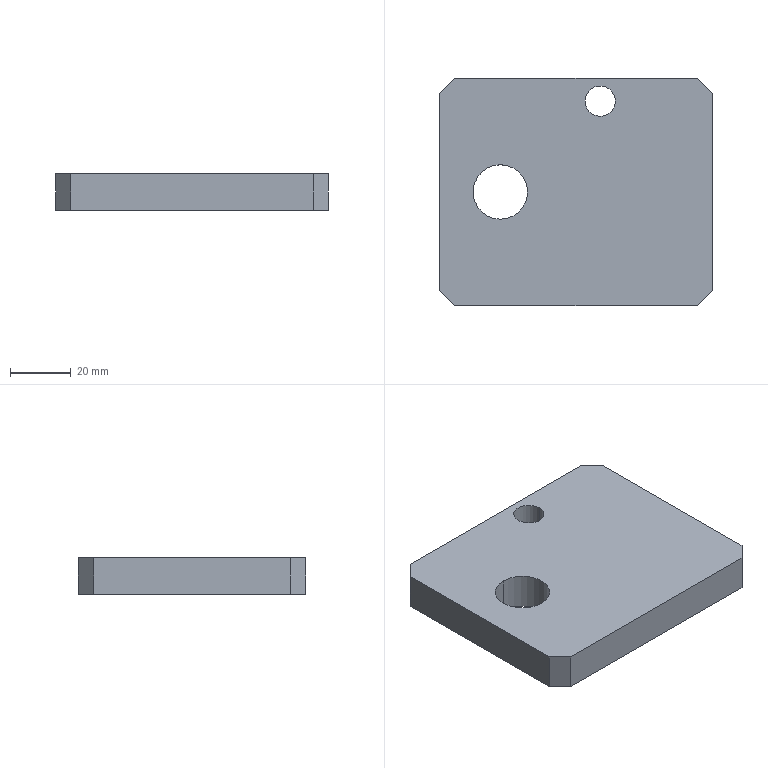Part | STEP file | [18] | 1 solid | 14 faces | box 90 x 75 x 12 mm | volume 76404 mm3 | plane 10 | cylinder 4 | commonest cylinder face diameters 10 x2 18 x2
STEP:
#1=CARTESIAN_POINT('',(20.,46.5,12.));
#2=VERTEX_POINT('',#1);
#3=CARTESIAN_POINT('',(20.,28.5,12.));
#4=VERTEX_POINT('',#3);
#5=CARTESIAN_POINT('',(20.,37.5,12.));
#6=DIRECTION('',(0.,0.,-1.));
#7=DIRECTION('',(0.,-1.,0.));
#8=AXIS2_PLACEMENT_3D('',#5,#6,#7);
#9=CIRCLE('',#8,9.);
#10=EDGE_CURVE('',#2,#4,#9,.T.);
#11=ORIENTED_EDGE('',*,*,#10,.F.);
#12=CARTESIAN_POINT('',(20.,46.5,0.));
#13=VERTEX_POINT('',#12);
#14=CARTESIAN_POINT('',(20.,46.5,12.));
#15=DIRECTION('',(0.,0.,-1.));
#16=VECTOR('',#15,1000.);
#17=LINE('',#14,#16);
#18=EDGE_CURVE('',#2,#13,#17,.T.);
#19=ORIENTED_EDGE('',*,*,#18,.T.);
#20=CARTESIAN_POINT('',(20.,28.5,0.));
#21=VERTEX_POINT('',#20);
#22=CARTESIAN_POINT('',(20.,37.5,0.));
#23=DIRECTION('',(0.,0.,1.));
#24=DIRECTION('',(0.,1.,0.));
#25=AXIS2_PLACEMENT_3D('',#22,#23,#24);
#26=CIRCLE('',#25,9.);
#27=EDGE_CURVE('',#21,#13,#26,.T.);
#28=ORIENTED_EDGE('',*,*,#27,.F.);
#29=CARTESIAN_POINT('',(20.,28.5,12.));
#30=DIRECTION('',(0.,0.,-1.));
#31=VECTOR('',#30,1000.);
#32=LINE('',#29,#31);
#33=EDGE_CURVE('',#4,#21,#32,.T.);
#34=ORIENTED_EDGE('',*,*,#33,.F.);
#35=EDGE_LOOP('',(#11,#19,#28,#34));
#36=FACE_OUTER_BOUND('',#35,.T.);
#37=CARTESIAN_POINT('',(20.,37.5,12.));
#38=DIRECTION('',(0.,0.,-1.));
#39=DIRECTION('',(0.,-1.,0.));
#40=AXIS2_PLACEMENT_3D('',#37,#38,#39);
#41=CYLINDRICAL_SURFACE('',#40,9.);
#42=ADVANCED_FACE('',(#36),#41,.F.);
#43=CARTESIAN_POINT('',(58.,67.5,0.));
#44=VERTEX_POINT('',#43);
#45=CARTESIAN_POINT('',(48.,67.5,0.));
#46=VERTEX_POINT('',#45);
#47=CARTESIAN_POINT('',(53.,67.5,0.));
#48=DIRECTION('',(0.,0.,1.));
#49=DIRECTION('',(-1.,0.,0.));
#50=AXIS2_PLACEMENT_3D('',#47,#48,#49);
#51=CIRCLE('',#50,5.);
#52=EDGE_CURVE('',#44,#46,#51,.T.);
#53=ORIENTED_EDGE('',*,*,#52,.F.);
#54=CARTESIAN_POINT('',(58.,67.5,12.));
#55=VERTEX_POINT('',#54);
#56=CARTESIAN_POINT('',(58.,67.5,0.));
#57=DIRECTION('',(0.,0.,1.));
#58=VECTOR('',#57,1000.);
#59=LINE('',#56,#58);
#60=EDGE_CURVE('',#44,#55,#59,.T.);
#61=ORIENTED_EDGE('',*,*,#60,.T.);
#62=CARTESIAN_POINT('',(48.,67.5,12.));
#63=VERTEX_POINT('',#62);
#64=CARTESIAN_POINT('',(53.,67.5,12.));
#65=DIRECTION('',(0.,0.,-1.));
#66=DIRECTION('',(1.,0.,0.));
#67=AXIS2_PLACEMENT_3D('',#64,#65,#66);
#68=CIRCLE('',#67,5.);
#69=EDGE_CURVE('',#63,#55,#68,.T.);
#70=ORIENTED_EDGE('',*,*,#69,.F.);
#71=CARTESIAN_POINT('',(48.,67.5,0.));
#72=DIRECTION('',(0.,0.,1.));
#73=VECTOR('',#72,1000.);
#74=LINE('',#71,#73);
#75=EDGE_CURVE('',#46,#63,#74,.T.);
#76=ORIENTED_EDGE('',*,*,#75,.F.);
#77=EDGE_LOOP('',(#53,#61,#70,#76));
#78=FACE_OUTER_BOUND('',#77,.T.);
#79=CARTESIAN_POINT('',(53.,67.5,0.));
#80=DIRECTION('',(0.,0.,1.));
#81=DIRECTION('',(-1.,0.,0.));
#82=AXIS2_PLACEMENT_3D('',#79,#80,#81);
#83=CYLINDRICAL_SURFACE('',#82,5.);
#84=ADVANCED_FACE('',(#78),#83,.F.);
#85=CARTESIAN_POINT('',(20.,37.5,12.));
#86=DIRECTION('',(0.,0.,-1.));
#87=DIRECTION('',(0.,-1.,0.));
#88=AXIS2_PLACEMENT_3D('',#85,#86,#87);
#89=CIRCLE('',#88,9.);
#90=EDGE_CURVE('',#4,#2,#89,.T.);
#91=ORIENTED_EDGE('',*,*,#90,.T.);
#92=ORIENTED_EDGE('',*,*,#10,.T.);
#93=EDGE_LOOP('',(#91,#92));
#94=FACE_BOUND('',#93,.T.);
#95=ORIENTED_EDGE('',*,*,#69,.T.);
#96=CARTESIAN_POINT('',(53.,67.5,12.));
#97=DIRECTION('',(0.,0.,-1.));
#98=DIRECTION('',(1.,0.,0.));
#99=AXIS2_PLACEMENT_3D('',#96,#97,#98);
#100=CIRCLE('',#99,5.);
#101=EDGE_CURVE('',#55,#63,#100,.T.);
#102=ORIENTED_EDGE('',*,*,#101,.T.);
#103=EDGE_LOOP('',(#95,#102));
#104=FACE_BOUND('',#103,.T.);
#105=CARTESIAN_POINT('',(5.,75.,12.));
#106=VERTEX_POINT('',#105);
#107=CARTESIAN_POINT('',(85.,75.,12.));
#108=VERTEX_POINT('',#107);
#109=CARTESIAN_POINT('',(45.,75.,12.));
#110=DIRECTION('',(1.,0.,0.));
#111=VECTOR('',#110,1000.);
#112=LINE('',#109,#111);
#113=EDGE_CURVE('',#106,#108,#112,.T.);
#114=ORIENTED_EDGE('',*,*,#113,.F.);
#115=CARTESIAN_POINT('',(0.,70.,12.));
#116=VERTEX_POINT('',#115);
#117=CARTESIAN_POINT('',(6.25,76.25,12.));
#118=DIRECTION('',(-0.7071,-0.7071,0.));
#119=VECTOR('',#118,1000.);
#120=LINE('',#117,#119);
#121=EDGE_CURVE('',#106,#116,#120,.T.);
#122=ORIENTED_EDGE('',*,*,#121,.T.);
#123=CARTESIAN_POINT('',(0.,5.,12.));
#124=VERTEX_POINT('',#123);
#125=CARTESIAN_POINT('',(0.,37.5,12.));
#126=DIRECTION('',(0.,1.,0.));
#127=VECTOR('',#126,1000.);
#128=LINE('',#125,#127);
#129=EDGE_CURVE('',#124,#116,#128,.T.);
#130=ORIENTED_EDGE('',*,*,#129,.F.);
#131=CARTESIAN_POINT('',(5.,0.,12.));
#132=VERTEX_POINT('',#131);
#133=CARTESIAN_POINT('',(6.25,-1.25,12.));
#134=DIRECTION('',(0.7071,-0.7071,0.));
#135=VECTOR('',#134,1000.);
#136=LINE('',#133,#135);
#137=EDGE_CURVE('',#124,#132,#136,.T.);
#138=ORIENTED_EDGE('',*,*,#137,.T.);
#139=CARTESIAN_POINT('',(85.,0.,12.));
#140=VERTEX_POINT('',#139);
#141=CARTESIAN_POINT('',(45.,0.,12.));
#142=DIRECTION('',(-1.,0.,0.));
#143=VECTOR('',#142,1000.);
#144=LINE('',#141,#143);
#145=EDGE_CURVE('',#140,#132,#144,.T.);
#146=ORIENTED_EDGE('',*,*,#145,.F.);
#147=CARTESIAN_POINT('',(90.,5.,12.));
#148=VERTEX_POINT('',#147);
#149=CARTESIAN_POINT('',(83.75,-1.25,12.));
#150=DIRECTION('',(0.7071,0.7071,0.));
#151=VECTOR('',#150,1000.);
#152=LINE('',#149,#151);
#153=EDGE_CURVE('',#140,#148,#152,.T.);
#154=ORIENTED_EDGE('',*,*,#153,.T.);
#155=CARTESIAN_POINT('',(90.,70.,12.));
#156=VERTEX_POINT('',#155);
#157=CARTESIAN_POINT('',(90.,37.5,12.));
#158=DIRECTION('',(0.,-1.,0.));
#159=VECTOR('',#158,1000.);
#160=LINE('',#157,#159);
#161=EDGE_CURVE('',#156,#148,#160,.T.);
#162=ORIENTED_EDGE('',*,*,#161,.F.);
#163=CARTESIAN_POINT('',(83.75,76.25,12.));
#164=DIRECTION('',(-0.7071,0.7071,0.));
#165=VECTOR('',#164,1000.);
#166=LINE('',#163,#165);
#167=EDGE_CURVE('',#156,#108,#166,.T.);
#168=ORIENTED_EDGE('',*,*,#167,.T.);
#169=EDGE_LOOP('',(#114,#122,#130,#138,#146,#154,#162,#168));
#170=FACE_OUTER_BOUND('',#169,.T.);
#171=CARTESIAN_POINT('',(45.,37.5,12.));
#172=DIRECTION('',(0.,0.,1.));
#173=DIRECTION('',(0.,1.,0.));
#174=AXIS2_PLACEMENT_3D('',#171,#172,#173);
#175=PLANE('',#174);
#176=ADVANCED_FACE('',(#94,#104,#170),#175,.T.);
#177=CARTESIAN_POINT('',(90.,5.,0.));
#178=VERTEX_POINT('',#177);
#179=CARTESIAN_POINT('',(90.,70.,0.));
#180=VERTEX_POINT('',#179);
#181=CARTESIAN_POINT('',(90.,37.5,0.));
#182=DIRECTION('',(0.,1.,0.));
#183=VECTOR('',#182,1000.);
#184=LINE('',#181,#183);
#185=EDGE_CURVE('',#178,#180,#184,.T.);
#186=ORIENTED_EDGE('',*,*,#185,.T.);
#187=CARTESIAN_POINT('',(90.,70.,0.));
#188=DIRECTION('',(0.,0.,1.));
#189=VECTOR('',#188,1000.);
#190=LINE('',#187,#189);
#191=EDGE_CURVE('',#180,#156,#190,.T.);
#192=ORIENTED_EDGE('',*,*,#191,.T.);
#193=ORIENTED_EDGE('',*,*,#161,.T.);
#194=CARTESIAN_POINT('',(90.,5.,0.));
#195=DIRECTION('',(0.,0.,-1.));
#196=VECTOR('',#195,1000.);
#197=LINE('',#194,#196);
#198=EDGE_CURVE('',#148,#178,#197,.T.);
#199=ORIENTED_EDGE('',*,*,#198,.T.);
#200=EDGE_LOOP('',(#186,#192,#193,#199));
#201=FACE_OUTER_BOUND('',#200,.T.);
#202=CARTESIAN_POINT('',(90.,37.5,0.));
#203=DIRECTION('',(1.,0.,0.));
#204=DIRECTION('',(0.,0.,-1.));
#205=AXIS2_PLACEMENT_3D('',#202,#203,#204);
#206=PLANE('',#205);
#207=ADVANCED_FACE('',(#201),#206,.T.);
#208=ORIENTED_EDGE('',*,*,#145,.T.);
#209=CARTESIAN_POINT('',(5.,0.,0.));
#210=VERTEX_POINT('',#209);
#211=CARTESIAN_POINT('',(5.,0.,0.));
#212=DIRECTION('',(0.,0.,-1.));
#213=VECTOR('',#212,1000.);
#214=LINE('',#211,#213);
#215=EDGE_CURVE('',#132,#210,#214,.T.);
#216=ORIENTED_EDGE('',*,*,#215,.T.);
#217=CARTESIAN_POINT('',(85.,0.,0.));
#218=VERTEX_POINT('',#217);
#219=CARTESIAN_POINT('',(45.,0.,0.));
#220=DIRECTION('',(1.,0.,0.));
#221=VECTOR('',#220,1000.);
#222=LINE('',#219,#221);
#223=EDGE_CURVE('',#210,#218,#222,.T.);
#224=ORIENTED_EDGE('',*,*,#223,.T.);
#225=CARTESIAN_POINT('',(85.,0.,0.));
#226=DIRECTION('',(0.,0.,1.));
#227=VECTOR('',#226,1000.);
#228=LINE('',#225,#227);
#229=EDGE_CURVE('',#218,#140,#228,.T.);
#230=ORIENTED_EDGE('',*,*,#229,.T.);
#231=EDGE_LOOP('',(#208,#216,#224,#230));
#232=FACE_OUTER_BOUND('',#231,.T.);
#233=CARTESIAN_POINT('',(45.,0.,0.));
#234=DIRECTION('',(0.,-1.,0.));
#235=DIRECTION('',(0.,0.,1.));
#236=AXIS2_PLACEMENT_3D('',#233,#234,#235);
#237=PLANE('',#236);
#238=ADVANCED_FACE('',(#232),#237,.T.);
#239=ORIENTED_EDGE('',*,*,#129,.T.);
#240=CARTESIAN_POINT('',(0.,70.,0.));
#241=VERTEX_POINT('',#240);
#242=CARTESIAN_POINT('',(0.,70.,0.));
#243=DIRECTION('',(0.,0.,-1.));
#244=VECTOR('',#243,1000.);
#245=LINE('',#242,#244);
#246=EDGE_CURVE('',#116,#241,#245,.T.);
#247=ORIENTED_EDGE('',*,*,#246,.T.);
#248=CARTESIAN_POINT('',(0.,5.,0.));
#249=VERTEX_POINT('',#248);
#250=CARTESIAN_POINT('',(0.,37.5,0.));
#251=DIRECTION('',(0.,-1.,0.));
#252=VECTOR('',#251,1000.);
#253=LINE('',#250,#252);
#254=EDGE_CURVE('',#241,#249,#253,.T.);
#255=ORIENTED_EDGE('',*,*,#254,.T.);
#256=CARTESIAN_POINT('',(0.,5.,0.));
#257=DIRECTION('',(0.,0.,1.));
#258=VECTOR('',#257,1000.);
#259=LINE('',#256,#258);
#260=EDGE_CURVE('',#249,#124,#259,.T.);
#261=ORIENTED_EDGE('',*,*,#260,.T.);
#262=EDGE_LOOP('',(#239,#247,#255,#261));
#263=FACE_OUTER_BOUND('',#262,.T.);
#264=CARTESIAN_POINT('',(0.,37.5,0.));
#265=DIRECTION('',(-1.,0.,0.));
#266=DIRECTION('',(0.,0.,1.));
#267=AXIS2_PLACEMENT_3D('',#264,#265,#266);
#268=PLANE('',#267);
#269=ADVANCED_FACE('',(#263),#268,.T.);
#270=ORIENTED_EDGE('',*,*,#27,.T.);
#271=CARTESIAN_POINT('',(20.,37.5,0.));
#272=DIRECTION('',(0.,0.,1.));
#273=DIRECTION('',(0.,1.,0.));
#274=AXIS2_PLACEMENT_3D('',#271,#272,#273);
#275=CIRCLE('',#274,9.);
#276=EDGE_CURVE('',#13,#21,#275,.T.);
#277=ORIENTED_EDGE('',*,*,#276,.T.);
#278=EDGE_LOOP('',(#270,#277));
#279=FACE_BOUND('',#278,.T.);
#280=CARTESIAN_POINT('',(53.,67.5,0.));
#281=DIRECTION('',(0.,0.,1.));
#282=DIRECTION('',(-1.,0.,0.));
#283=AXIS2_PLACEMENT_3D('',#280,#281,#282);
#284=CIRCLE('',#283,5.);
#285=EDGE_CURVE('',#46,#44,#284,.T.);
#286=ORIENTED_EDGE('',*,*,#285,.T.);
#287=ORIENTED_EDGE('',*,*,#52,.T.);
#288=EDGE_LOOP('',(#286,#287));
#289=FACE_BOUND('',#288,.T.);
#290=ORIENTED_EDGE('',*,*,#254,.F.);
#291=CARTESIAN_POINT('',(5.,75.,0.));
#292=VERTEX_POINT('',#291);
#293=CARTESIAN_POINT('',(6.25,76.25,0.));
#294=DIRECTION('',(0.7071,0.7071,0.));
#295=VECTOR('',#294,1000.);
#296=LINE('',#293,#295);
#297=EDGE_CURVE('',#241,#292,#296,.T.);
#298=ORIENTED_EDGE('',*,*,#297,.T.);
#299=CARTESIAN_POINT('',(85.,75.,0.));
#300=VERTEX_POINT('',#299);
#301=CARTESIAN_POINT('',(45.,75.,0.));
#302=DIRECTION('',(-1.,0.,0.));
#303=VECTOR('',#302,1000.);
#304=LINE('',#301,#303);
#305=EDGE_CURVE('',#300,#292,#304,.T.);
#306=ORIENTED_EDGE('',*,*,#305,.F.);
#307=CARTESIAN_POINT('',(83.75,76.25,0.));
#308=DIRECTION('',(0.7071,-0.7071,0.));
#309=VECTOR('',#308,1000.);
#310=LINE('',#307,#309);
#311=EDGE_CURVE('',#300,#180,#310,.T.);
#312=ORIENTED_EDGE('',*,*,#311,.T.);
#313=ORIENTED_EDGE('',*,*,#185,.F.);
#314=CARTESIAN_POINT('',(83.75,-1.25,0.));
#315=DIRECTION('',(-0.7071,-0.7071,0.));
#316=VECTOR('',#315,1000.);
#317=LINE('',#314,#316);
#318=EDGE_CURVE('',#178,#218,#317,.T.);
#319=ORIENTED_EDGE('',*,*,#318,.T.);
#320=ORIENTED_EDGE('',*,*,#223,.F.);
#321=CARTESIAN_POINT('',(6.25,-1.25,0.));
#322=DIRECTION('',(-0.7071,0.7071,0.));
#323=VECTOR('',#322,1000.);
#324=LINE('',#321,#323);
#325=EDGE_CURVE('',#210,#249,#324,.T.);
#326=ORIENTED_EDGE('',*,*,#325,.T.);
#327=EDGE_LOOP('',(#290,#298,#306,#312,#313,#319,#320,#326));
#328=FACE_OUTER_BOUND('',#327,.T.);
#329=CARTESIAN_POINT('',(45.,37.5,0.));
#330=DIRECTION('',(0.,0.,-1.));
#331=DIRECTION('',(0.,-1.,0.));
#332=AXIS2_PLACEMENT_3D('',#329,#330,#331);
#333=PLANE('',#332);
#334=ADVANCED_FACE('',(#279,#289,#328),#333,.T.);
#335=ORIENTED_EDGE('',*,*,#305,.T.);
#336=CARTESIAN_POINT('',(5.,75.,0.));
#337=DIRECTION('',(0.,0.,1.));
#338=VECTOR('',#337,1000.);
#339=LINE('',#336,#338);
#340=EDGE_CURVE('',#292,#106,#339,.T.);
#341=ORIENTED_EDGE('',*,*,#340,.T.);
#342=ORIENTED_EDGE('',*,*,#113,.T.);
#343=CARTESIAN_POINT('',(85.,75.,0.));
#344=DIRECTION('',(0.,0.,-1.));
#345=VECTOR('',#344,1000.);
#346=LINE('',#343,#345);
#347=EDGE_CURVE('',#108,#300,#346,.T.);
#348=ORIENTED_EDGE('',*,*,#347,.T.);
#349=EDGE_LOOP('',(#335,#341,#342,#348));
#350=FACE_OUTER_BOUND('',#349,.T.);
#351=CARTESIAN_POINT('',(45.,75.,0.));
#352=DIRECTION('',(0.,1.,0.));
#353=DIRECTION('',(0.,0.,-1.));
#354=AXIS2_PLACEMENT_3D('',#351,#352,#353);
#355=PLANE('',#354);
#356=ADVANCED_FACE('',(#350),#355,.T.);
#357=ORIENTED_EDGE('',*,*,#311,.F.);
#358=ORIENTED_EDGE('',*,*,#347,.F.);
#359=ORIENTED_EDGE('',*,*,#167,.F.);
#360=ORIENTED_EDGE('',*,*,#191,.F.);
#361=EDGE_LOOP('',(#357,#358,#359,#360));
#362=FACE_OUTER_BOUND('',#361,.T.);
#363=CARTESIAN_POINT('',(90.,70.,0.));
#364=DIRECTION('',(-0.7071,-0.7071,0.));
#365=DIRECTION('',(0.,0.,1.));
#366=AXIS2_PLACEMENT_3D('',#363,#364,#365);
#367=PLANE('',#366);
#368=ADVANCED_FACE('',(#362),#367,.F.);
#369=ORIENTED_EDGE('',*,*,#318,.F.);
#370=ORIENTED_EDGE('',*,*,#198,.F.);
#371=ORIENTED_EDGE('',*,*,#153,.F.);
#372=ORIENTED_EDGE('',*,*,#229,.F.);
#373=EDGE_LOOP('',(#369,#370,#371,#372));
#374=FACE_OUTER_BOUND('',#373,.T.);
#375=CARTESIAN_POINT('',(85.,0.,0.));
#376=DIRECTION('',(-0.7071,0.7071,0.));
#377=DIRECTION('',(0.,0.,1.));
#378=AXIS2_PLACEMENT_3D('',#375,#376,#377);
#379=PLANE('',#378);
#380=ADVANCED_FACE('',(#374),#379,.F.);
#381=ORIENTED_EDGE('',*,*,#297,.F.);
#382=ORIENTED_EDGE('',*,*,#246,.F.);
#383=ORIENTED_EDGE('',*,*,#121,.F.);
#384=ORIENTED_EDGE('',*,*,#340,.F.);
#385=EDGE_LOOP('',(#381,#382,#383,#384));
#386=FACE_OUTER_BOUND('',#385,.T.);
#387=CARTESIAN_POINT('',(5.,75.,0.));
#388=DIRECTION('',(0.7071,-0.7071,0.));
#389=DIRECTION('',(0.,0.,1.));
#390=AXIS2_PLACEMENT_3D('',#387,#388,#389);
#391=PLANE('',#390);
#392=ADVANCED_FACE('',(#386),#391,.F.);
#393=ORIENTED_EDGE('',*,*,#325,.F.);
#394=ORIENTED_EDGE('',*,*,#215,.F.);
#395=ORIENTED_EDGE('',*,*,#137,.F.);
#396=ORIENTED_EDGE('',*,*,#260,.F.);
#397=EDGE_LOOP('',(#393,#394,#395,#396));
#398=FACE_OUTER_BOUND('',#397,.T.);
#399=CARTESIAN_POINT('',(0.,5.,0.));
#400=DIRECTION('',(0.7071,0.7071,0.));
#401=DIRECTION('',(0.,0.,1.));
#402=AXIS2_PLACEMENT_3D('',#399,#400,#401);
#403=PLANE('',#402);
#404=ADVANCED_FACE('',(#398),#403,.F.);
#405=ORIENTED_EDGE('',*,*,#60,.F.);
#406=ORIENTED_EDGE('',*,*,#285,.F.);
#407=ORIENTED_EDGE('',*,*,#75,.T.);
#408=ORIENTED_EDGE('',*,*,#101,.F.);
#409=EDGE_LOOP('',(#405,#406,#407,#408));
#410=FACE_OUTER_BOUND('',#409,.T.);
#411=CARTESIAN_POINT('',(53.,67.5,0.));
#412=DIRECTION('',(0.,0.,1.));
#413=DIRECTION('',(-1.,0.,0.));
#414=AXIS2_PLACEMENT_3D('',#411,#412,#413);
#415=CYLINDRICAL_SURFACE('',#414,5.);
#416=ADVANCED_FACE('',(#410),#415,.F.);
#417=ORIENTED_EDGE('',*,*,#18,.F.);
#418=ORIENTED_EDGE('',*,*,#90,.F.);
#419=ORIENTED_EDGE('',*,*,#33,.T.);
#420=ORIENTED_EDGE('',*,*,#276,.F.);
#421=EDGE_LOOP('',(#417,#418,#419,#420));
#422=FACE_OUTER_BOUND('',#421,.T.);
#423=CARTESIAN_POINT('',(20.,37.5,12.));
#424=DIRECTION('',(0.,0.,-1.));
#425=DIRECTION('',(0.,-1.,0.));
#426=AXIS2_PLACEMENT_3D('',#423,#424,#425);
#427=CYLINDRICAL_SURFACE('',#426,9.);
#428=ADVANCED_FACE('',(#422),#427,.F.);
#429=CLOSED_SHELL('',(#42,#84,#176,#207,#238,#269,#334,#356,#368,#380,#392,#404,#416,#428));
#430=MANIFOLD_SOLID_BREP('',#429);
#431=CARTESIAN_POINT('',(0.,0.,0.));
#432=DIRECTION('',(0.,0.,1.));
#433=DIRECTION('',(1.,0.,0.));
#434=AXIS2_PLACEMENT_3D('',#431,#432,#433);
#435=(LENGTH_UNIT()NAMED_UNIT(*)SI_UNIT(.MILLI.,.METRE.));
#436=UNCERTAINTY_MEASURE_WITH_UNIT(LENGTH_MEASURE(0.00001),#435,'','');
#437=(NAMED_UNIT(*)PLANE_ANGLE_UNIT()SI_UNIT($,.RADIAN.));
#438=(NAMED_UNIT(*)SI_UNIT($,.STERADIAN.)SOLID_ANGLE_UNIT());
#439=(GEOMETRIC_REPRESENTATION_CONTEXT(3)GLOBAL_UNCERTAINTY_ASSIGNED_CONTEXT((#436))GLOBAL_UNIT_ASSIGNED_CONTEXT((#435,#437,#438))REPRESENTATION_CONTEXT('',''));
#440=ADVANCED_BREP_SHAPE_REPRESENTATION('',(#430,#434),#439);